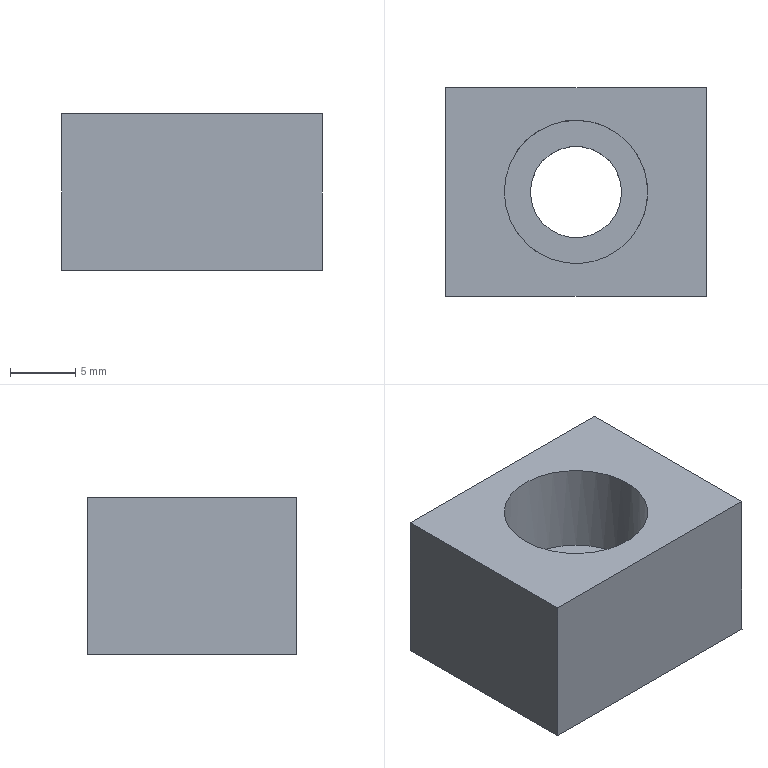Part | STEP file | gslz 2016.10.28-6_id698_x_t | 1 solid | 9 faces | box 20 x 16 x 12 mm | volume 2982 mm3 | plane 7 | cylinder 2 | commonest cylinder face diameters 7 x1 11 x1
STEP:
#1=CARTESIAN_POINT('',(90.7,158.,45.));
#2=VERTEX_POINT('',#1);
#3=CARTESIAN_POINT('',(90.7,142.,45.));
#4=VERTEX_POINT('',#3);
#5=CARTESIAN_POINT('',(90.7,150.,45.));
#6=DIRECTION('',(0.0000204,-1.,0.));
#7=VECTOR('',#6,1.);
#8=LINE('',#5,#7);
#9=EDGE_CURVE('',#2,#4,#8,.T.);
#10=ORIENTED_EDGE('',*,*,#9,.T.);
#11=CARTESIAN_POINT('',(110.7,142.,45.));
#12=VERTEX_POINT('',#11);
#13=CARTESIAN_POINT('',(102.7,142.,45.));
#14=DIRECTION('',(1.,0.0000204,0.));
#15=VECTOR('',#14,1.);
#16=LINE('',#13,#15);
#17=EDGE_CURVE('',#4,#12,#16,.T.);
#18=ORIENTED_EDGE('',*,*,#17,.T.);
#19=CARTESIAN_POINT('',(110.7,158.,45.));
#20=VERTEX_POINT('',#19);
#21=CARTESIAN_POINT('',(110.7,150.,45.));
#22=DIRECTION('',(-0.0000204,1.,0.));
#23=VECTOR('',#22,1.);
#24=LINE('',#21,#23);
#25=EDGE_CURVE('',#12,#20,#24,.T.);
#26=ORIENTED_EDGE('',*,*,#25,.T.);
#27=CARTESIAN_POINT('',(102.7,158.,45.));
#28=DIRECTION('',(-1.,-0.0000204,0.));
#29=VECTOR('',#28,1.);
#30=LINE('',#27,#29);
#31=EDGE_CURVE('',#20,#2,#30,.T.);
#32=ORIENTED_EDGE('',*,*,#31,.T.);
#33=EDGE_LOOP('',(#10,#18,#26,#32));
#34=FACE_BOUND('',#33,.T.);
#35=CARTESIAN_POINT('',(95.2,150.,45.));
#36=VERTEX_POINT('',#35);
#37=CARTESIAN_POINT('',(100.7,150.,45.));
#38=DIRECTION('',(0.,0.,1.));
#39=DIRECTION('',(-1.,0.,0.));
#40=AXIS2_PLACEMENT_3D('',#37,#38,#39);
#41=CIRCLE('',#40,5.5);
#42=EDGE_CURVE('',#36,#36,#41,.T.);
#43=ORIENTED_EDGE('',*,*,#42,.F.);
#44=EDGE_LOOP('',(#43));
#45=FACE_BOUND('',#44,.T.);
#46=CARTESIAN_POINT('',(102.7,150.,45.));
#47=DIRECTION('',(0.,0.,1.));
#48=DIRECTION('',(0.0000204,-1.,0.));
#49=AXIS2_PLACEMENT_3D('',#46,#47,#48);
#50=PLANE('',#49);
#51=ADVANCED_FACE('',(#34,#45),#50,.T.);
#52=CARTESIAN_POINT('',(90.7,158.,33.));
#53=VERTEX_POINT('',#52);
#54=CARTESIAN_POINT('',(90.7,158.,35.));
#55=DIRECTION('',(0.,0.,1.));
#56=VECTOR('',#55,1.);
#57=LINE('',#54,#56);
#58=EDGE_CURVE('',#53,#2,#57,.T.);
#59=ORIENTED_EDGE('',*,*,#58,.F.);
#60=CARTESIAN_POINT('',(90.7,142.,33.));
#61=VERTEX_POINT('',#60);
#62=CARTESIAN_POINT('',(90.7,150.,33.));
#63=DIRECTION('',(-0.0000204,1.,0.));
#64=VECTOR('',#63,1.);
#65=LINE('',#62,#64);
#66=EDGE_CURVE('',#61,#53,#65,.T.);
#67=ORIENTED_EDGE('',*,*,#66,.F.);
#68=CARTESIAN_POINT('',(90.7,142.,35.));
#69=DIRECTION('',(0.,0.,1.));
#70=VECTOR('',#69,1.);
#71=LINE('',#68,#70);
#72=EDGE_CURVE('',#61,#4,#71,.T.);
#73=ORIENTED_EDGE('',*,*,#72,.T.);
#74=ORIENTED_EDGE('',*,*,#9,.F.);
#75=EDGE_LOOP('',(#59,#67,#73,#74));
#76=FACE_OUTER_BOUND('',#75,.T.);
#77=CARTESIAN_POINT('',(90.7,150.,35.));
#78=DIRECTION('',(-1.,-0.0000204,0.));
#79=DIRECTION('',(0.,0.,1.));
#80=AXIS2_PLACEMENT_3D('',#77,#78,#79);
#81=PLANE('',#80);
#82=ADVANCED_FACE('',(#76),#81,.T.);
#83=ORIENTED_EDGE('',*,*,#72,.F.);
#84=CARTESIAN_POINT('',(110.7,142.,33.));
#85=VERTEX_POINT('',#84);
#86=CARTESIAN_POINT('',(102.7,142.,33.));
#87=DIRECTION('',(-1.,-0.0000204,0.));
#88=VECTOR('',#87,1.);
#89=LINE('',#86,#88);
#90=EDGE_CURVE('',#85,#61,#89,.T.);
#91=ORIENTED_EDGE('',*,*,#90,.F.);
#92=CARTESIAN_POINT('',(110.7,142.,35.));
#93=DIRECTION('',(0.,0.,1.));
#94=VECTOR('',#93,1.);
#95=LINE('',#92,#94);
#96=EDGE_CURVE('',#85,#12,#95,.T.);
#97=ORIENTED_EDGE('',*,*,#96,.T.);
#98=ORIENTED_EDGE('',*,*,#17,.F.);
#99=EDGE_LOOP('',(#83,#91,#97,#98));
#100=FACE_OUTER_BOUND('',#99,.T.);
#101=CARTESIAN_POINT('',(102.7,142.,35.));
#102=DIRECTION('',(0.0000204,-1.,0.));
#103=DIRECTION('',(0.,0.,-1.));
#104=AXIS2_PLACEMENT_3D('',#101,#102,#103);
#105=PLANE('',#104);
#106=ADVANCED_FACE('',(#100),#105,.T.);
#107=ORIENTED_EDGE('',*,*,#96,.F.);
#108=CARTESIAN_POINT('',(110.7,158.,33.));
#109=VERTEX_POINT('',#108);
#110=CARTESIAN_POINT('',(110.7,150.,33.));
#111=DIRECTION('',(0.0000204,-1.,0.));
#112=VECTOR('',#111,1.);
#113=LINE('',#110,#112);
#114=EDGE_CURVE('',#109,#85,#113,.T.);
#115=ORIENTED_EDGE('',*,*,#114,.F.);
#116=CARTESIAN_POINT('',(110.7,158.,35.));
#117=DIRECTION('',(0.,0.,1.));
#118=VECTOR('',#117,1.);
#119=LINE('',#116,#118);
#120=EDGE_CURVE('',#109,#20,#119,.T.);
#121=ORIENTED_EDGE('',*,*,#120,.T.);
#122=ORIENTED_EDGE('',*,*,#25,.F.);
#123=EDGE_LOOP('',(#107,#115,#121,#122));
#124=FACE_OUTER_BOUND('',#123,.T.);
#125=CARTESIAN_POINT('',(110.7,150.,35.));
#126=DIRECTION('',(1.,0.0000204,0.));
#127=DIRECTION('',(0.,0.,-1.));
#128=AXIS2_PLACEMENT_3D('',#125,#126,#127);
#129=PLANE('',#128);
#130=ADVANCED_FACE('',(#124),#129,.T.);
#131=CARTESIAN_POINT('',(104.2,150.,33.));
#132=VERTEX_POINT('',#131);
#133=CARTESIAN_POINT('',(100.7,150.,33.));
#134=DIRECTION('',(0.,0.,1.));
#135=DIRECTION('',(1.,0.,0.));
#136=AXIS2_PLACEMENT_3D('',#133,#134,#135);
#137=CIRCLE('',#136,3.5);
#138=EDGE_CURVE('',#132,#132,#137,.T.);
#139=ORIENTED_EDGE('',*,*,#138,.T.);
#140=EDGE_LOOP('',(#139));
#141=FACE_BOUND('',#140,.T.);
#142=CARTESIAN_POINT('',(102.7,158.,33.));
#143=DIRECTION('',(1.,0.0000204,0.));
#144=VECTOR('',#143,1.);
#145=LINE('',#142,#144);
#146=EDGE_CURVE('',#53,#109,#145,.T.);
#147=ORIENTED_EDGE('',*,*,#146,.T.);
#148=ORIENTED_EDGE('',*,*,#114,.T.);
#149=ORIENTED_EDGE('',*,*,#90,.T.);
#150=ORIENTED_EDGE('',*,*,#66,.T.);
#151=EDGE_LOOP('',(#147,#148,#149,#150));
#152=FACE_BOUND('',#151,.T.);
#153=CARTESIAN_POINT('',(102.7,150.,33.));
#154=DIRECTION('',(0.,0.,-1.));
#155=DIRECTION('',(-0.0000204,1.,0.));
#156=AXIS2_PLACEMENT_3D('',#153,#154,#155);
#157=PLANE('',#156);
#158=ADVANCED_FACE('',(#141,#152),#157,.T.);
#159=ORIENTED_EDGE('',*,*,#146,.F.);
#160=ORIENTED_EDGE('',*,*,#58,.T.);
#161=ORIENTED_EDGE('',*,*,#31,.F.);
#162=ORIENTED_EDGE('',*,*,#120,.F.);
#163=EDGE_LOOP('',(#159,#160,#161,#162));
#164=FACE_OUTER_BOUND('',#163,.T.);
#165=CARTESIAN_POINT('',(102.7,158.,35.));
#166=DIRECTION('',(-0.0000204,1.,0.));
#167=DIRECTION('',(0.,0.,1.));
#168=AXIS2_PLACEMENT_3D('',#165,#166,#167);
#169=PLANE('',#168);
#170=ADVANCED_FACE('',(#164),#169,.T.);
#171=ORIENTED_EDGE('',*,*,#138,.F.);
#172=EDGE_LOOP('',(#171));
#173=FACE_BOUND('',#172,.T.);
#174=CARTESIAN_POINT('',(104.2,150.,38.));
#175=VERTEX_POINT('',#174);
#176=CARTESIAN_POINT('',(100.7,150.,38.));
#177=DIRECTION('',(0.,0.,-1.));
#178=DIRECTION('',(1.,0.,0.));
#179=AXIS2_PLACEMENT_3D('',#176,#177,#178);
#180=CIRCLE('',#179,3.5);
#181=EDGE_CURVE('',#175,#175,#180,.T.);
#182=ORIENTED_EDGE('',*,*,#181,.F.);
#183=EDGE_LOOP('',(#182));
#184=FACE_BOUND('',#183,.T.);
#185=CARTESIAN_POINT('',(100.7,150.,32.));
#186=DIRECTION('',(0.,0.,-1.));
#187=DIRECTION('',(-1.,0.,0.));
#188=AXIS2_PLACEMENT_3D('',#185,#186,#187);
#189=CYLINDRICAL_SURFACE('',#188,3.5);
#190=ADVANCED_FACE('',(#173,#184),#189,.F.);
#191=ORIENTED_EDGE('',*,*,#181,.T.);
#192=EDGE_LOOP('',(#191));
#193=FACE_BOUND('',#192,.T.);
#194=CARTESIAN_POINT('',(106.2,150.,38.));
#195=VERTEX_POINT('',#194);
#196=CARTESIAN_POINT('',(100.7,150.,38.));
#197=DIRECTION('',(0.,0.,-1.));
#198=DIRECTION('',(1.,0.,0.));
#199=AXIS2_PLACEMENT_3D('',#196,#197,#198);
#200=CIRCLE('',#199,5.5);
#201=EDGE_CURVE('',#195,#195,#200,.T.);
#202=ORIENTED_EDGE('',*,*,#201,.F.);
#203=EDGE_LOOP('',(#202));
#204=FACE_BOUND('',#203,.T.);
#205=CARTESIAN_POINT('',(100.7,150.,38.));
#206=DIRECTION('',(0.,0.,-1.));
#207=DIRECTION('',(-1.,0.,0.));
#208=AXIS2_PLACEMENT_3D('',#205,#206,#207);
#209=PLANE('',#208);
#210=ADVANCED_FACE('',(#193,#204),#209,.F.);
#211=ORIENTED_EDGE('',*,*,#201,.T.);
#212=EDGE_LOOP('',(#211));
#213=FACE_BOUND('',#212,.T.);
#214=ORIENTED_EDGE('',*,*,#42,.T.);
#215=EDGE_LOOP('',(#214));
#216=FACE_BOUND('',#215,.T.);
#217=CARTESIAN_POINT('',(100.7,150.,47.));
#218=DIRECTION('',(0.,0.,-1.));
#219=DIRECTION('',(-1.,0.,0.));
#220=AXIS2_PLACEMENT_3D('',#217,#218,#219);
#221=CYLINDRICAL_SURFACE('',#220,5.5);
#222=ADVANCED_FACE('',(#213,#216),#221,.F.);
#223=CLOSED_SHELL('',(#51,#82,#106,#130,#158,#170,#190,#210,#222));
#224=MANIFOLD_SOLID_BREP('',#223);
#225=(LENGTH_UNIT()NAMED_UNIT(*)SI_UNIT(.MILLI.,.METRE.));
#226=UNCERTAINTY_MEASURE_WITH_UNIT(LENGTH_MEASURE(0.00002),#225,'','');
#227=(NAMED_UNIT(*)PLANE_ANGLE_UNIT()SI_UNIT($,.RADIAN.));
#228=PLANE_ANGLE_MEASURE_WITH_UNIT(PLANE_ANGLE_MEASURE(0.01745),#227);
#229=DIMENSIONAL_EXPONENTS(0.,0.,0.,0.,0.,0.,0.);
#230=(CONVERSION_BASED_UNIT('DEGREE',#228)NAMED_UNIT(#229)PLANE_ANGLE_UNIT());
#231=(NAMED_UNIT(*)SI_UNIT($,.STERADIAN.)SOLID_ANGLE_UNIT());
#232=(GEOMETRIC_REPRESENTATION_CONTEXT(3)GLOBAL_UNCERTAINTY_ASSIGNED_CONTEXT((#226))GLOBAL_UNIT_ASSIGNED_CONTEXT((#225,#230,#231))REPRESENTATION_CONTEXT('',''));
#233=ADVANCED_BREP_SHAPE_REPRESENTATION('',(#224),#232);